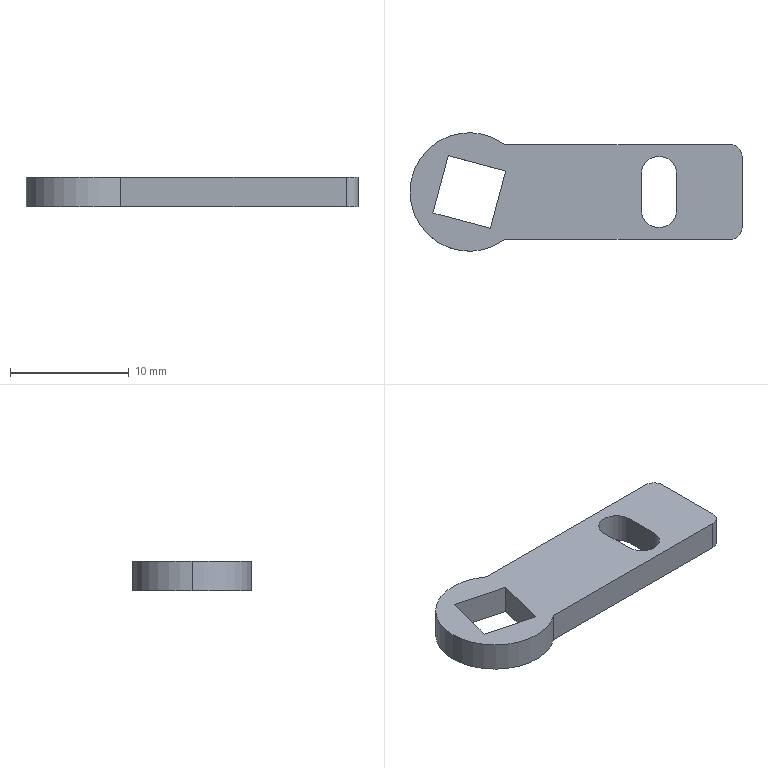Part | SolidWorks | features Extrusion 1, Fillet 1, ICE 1 | 1 solid | 17 faces | box 28 x 10 x 2.5 mm | volume 464.649 mm3 | plane 11 | cylinder 6 | commonest cylinder face diameters 2 x2 3 x2 10 x2
STEP:
#1=CARTESIAN_POINT('',(-5.,0.,1.25));
#2=VERTEX_POINT('',#1);
#3=CARTESIAN_POINT('',(3.,-4.,1.25));
#4=VERTEX_POINT('',#3);
#5=CARTESIAN_POINT('',(0.,0.,1.25));
#6=DIRECTION('',(0.,0.,1.));
#7=DIRECTION('',(1.,0.,0.));
#8=AXIS2_PLACEMENT_3D('',#5,#6,#7);
#9=CIRCLE('',#8,5.);
#10=EDGE_CURVE('',#2,#4,#9,.T.);
#11=ORIENTED_EDGE('',*,*,#10,.F.);
#12=CARTESIAN_POINT('',(-5.,0.,-1.25));
#13=VERTEX_POINT('',#12);
#14=CARTESIAN_POINT('',(-5.,0.,1.25));
#15=DIRECTION('',(0.,0.,-1.));
#16=VECTOR('',#15,1000.);
#17=LINE('',#14,#16);
#18=EDGE_CURVE('',#2,#13,#17,.T.);
#19=ORIENTED_EDGE('',*,*,#18,.T.);
#20=CARTESIAN_POINT('',(3.,-4.,-1.25));
#21=VERTEX_POINT('',#20);
#22=CARTESIAN_POINT('',(0.,0.,-1.25));
#23=DIRECTION('',(0.,0.,1.));
#24=DIRECTION('',(1.,0.,0.));
#25=AXIS2_PLACEMENT_3D('',#22,#23,#24);
#26=CIRCLE('',#25,5.);
#27=EDGE_CURVE('',#13,#21,#26,.T.);
#28=ORIENTED_EDGE('',*,*,#27,.T.);
#29=CARTESIAN_POINT('',(3.,-4.,1.25));
#30=DIRECTION('',(0.,0.,-1.));
#31=VECTOR('',#30,1000.);
#32=LINE('',#29,#31);
#33=EDGE_CURVE('',#4,#21,#32,.T.);
#34=ORIENTED_EDGE('',*,*,#33,.F.);
#35=EDGE_LOOP('',(#11,#19,#28,#34));
#36=FACE_OUTER_BOUND('',#35,.T.);
#37=CARTESIAN_POINT('',(0.,0.,1.25));
#38=DIRECTION('',(0.,0.,-1.));
#39=DIRECTION('',(-1.,0.,0.));
#40=AXIS2_PLACEMENT_3D('',#37,#38,#39);
#41=CYLINDRICAL_SURFACE('',#40,5.);
#42=ADVANCED_FACE('',(#36),#41,.T.);
#43=ORIENTED_EDGE('',*,*,#18,.F.);
#44=CARTESIAN_POINT('',(3.,4.,1.25));
#45=VERTEX_POINT('',#44);
#46=CARTESIAN_POINT('',(0.,0.,1.25));
#47=DIRECTION('',(0.,0.,1.));
#48=DIRECTION('',(1.,0.,0.));
#49=AXIS2_PLACEMENT_3D('',#46,#47,#48);
#50=CIRCLE('',#49,5.);
#51=EDGE_CURVE('',#45,#2,#50,.T.);
#52=ORIENTED_EDGE('',*,*,#51,.F.);
#53=CARTESIAN_POINT('',(3.,4.,-1.25));
#54=VERTEX_POINT('',#53);
#55=CARTESIAN_POINT('',(3.,4.,1.25));
#56=DIRECTION('',(0.,0.,-1.));
#57=VECTOR('',#56,1000.);
#58=LINE('',#55,#57);
#59=EDGE_CURVE('',#45,#54,#58,.T.);
#60=ORIENTED_EDGE('',*,*,#59,.T.);
#61=CARTESIAN_POINT('',(0.,0.,-1.25));
#62=DIRECTION('',(0.,0.,1.));
#63=DIRECTION('',(1.,0.,0.));
#64=AXIS2_PLACEMENT_3D('',#61,#62,#63);
#65=CIRCLE('',#64,5.);
#66=EDGE_CURVE('',#54,#13,#65,.T.);
#67=ORIENTED_EDGE('',*,*,#66,.T.);
#68=EDGE_LOOP('',(#43,#52,#60,#67));
#69=FACE_OUTER_BOUND('',#68,.T.);
#70=CARTESIAN_POINT('',(0.,0.,1.25));
#71=DIRECTION('',(0.,0.,-1.));
#72=DIRECTION('',(-1.,0.,0.));
#73=AXIS2_PLACEMENT_3D('',#70,#71,#72);
#74=CYLINDRICAL_SURFACE('',#73,5.);
#75=ADVANCED_FACE('',(#69),#74,.T.);
#76=CARTESIAN_POINT('',(22.,-4.,-1.25));
#77=VERTEX_POINT('',#76);
#78=CARTESIAN_POINT('',(3.,-4.,-1.25));
#79=DIRECTION('',(1.,0.,0.));
#80=VECTOR('',#79,1000.);
#81=LINE('',#78,#80);
#82=EDGE_CURVE('',#21,#77,#81,.T.);
#83=ORIENTED_EDGE('',*,*,#82,.T.);
#84=CARTESIAN_POINT('',(22.,-4.,1.25));
#85=VERTEX_POINT('',#84);
#86=CARTESIAN_POINT('',(22.,-4.,1.25));
#87=DIRECTION('',(0.,0.,1.));
#88=VECTOR('',#87,1000.);
#89=LINE('',#86,#88);
#90=EDGE_CURVE('',#77,#85,#89,.T.);
#91=ORIENTED_EDGE('',*,*,#90,.T.);
#92=CARTESIAN_POINT('',(3.,-4.,1.25));
#93=DIRECTION('',(1.,0.,0.));
#94=VECTOR('',#93,1000.);
#95=LINE('',#92,#94);
#96=EDGE_CURVE('',#4,#85,#95,.T.);
#97=ORIENTED_EDGE('',*,*,#96,.F.);
#98=ORIENTED_EDGE('',*,*,#33,.T.);
#99=EDGE_LOOP('',(#83,#91,#97,#98));
#100=FACE_OUTER_BOUND('',#99,.T.);
#101=CARTESIAN_POINT('',(3.,-4.,1.25));
#102=DIRECTION('',(0.,1.,0.));
#103=DIRECTION('',(0.,0.,1.));
#104=AXIS2_PLACEMENT_3D('',#101,#102,#103);
#105=PLANE('',#104);
#106=ADVANCED_FACE('',(#100),#105,.F.);
#107=CARTESIAN_POINT('',(23.,-3.,1.25));
#108=VERTEX_POINT('',#107);
#109=CARTESIAN_POINT('',(23.,3.,1.25));
#110=VERTEX_POINT('',#109);
#111=CARTESIAN_POINT('',(23.,4.,1.25));
#112=DIRECTION('',(0.,1.,0.));
#113=VECTOR('',#112,1000.);
#114=LINE('',#111,#113);
#115=EDGE_CURVE('',#108,#110,#114,.T.);
#116=ORIENTED_EDGE('',*,*,#115,.F.);
#117=CARTESIAN_POINT('',(23.,-3.,-1.25));
#118=VERTEX_POINT('',#117);
#119=CARTESIAN_POINT('',(23.,-3.,1.25));
#120=DIRECTION('',(0.,0.,-1.));
#121=VECTOR('',#120,1000.);
#122=LINE('',#119,#121);
#123=EDGE_CURVE('',#108,#118,#122,.T.);
#124=ORIENTED_EDGE('',*,*,#123,.T.);
#125=CARTESIAN_POINT('',(23.,3.,-1.25));
#126=VERTEX_POINT('',#125);
#127=CARTESIAN_POINT('',(23.,4.,-1.25));
#128=DIRECTION('',(0.,1.,0.));
#129=VECTOR('',#128,1000.);
#130=LINE('',#127,#129);
#131=EDGE_CURVE('',#118,#126,#130,.T.);
#132=ORIENTED_EDGE('',*,*,#131,.T.);
#133=CARTESIAN_POINT('',(23.,3.,1.25));
#134=DIRECTION('',(0.,0.,1.));
#135=VECTOR('',#134,1000.);
#136=LINE('',#133,#135);
#137=EDGE_CURVE('',#126,#110,#136,.T.);
#138=ORIENTED_EDGE('',*,*,#137,.T.);
#139=EDGE_LOOP('',(#116,#124,#132,#138));
#140=FACE_OUTER_BOUND('',#139,.T.);
#141=CARTESIAN_POINT('',(23.,4.,1.25));
#142=DIRECTION('',(-1.,0.,0.));
#143=DIRECTION('',(0.,0.,1.));
#144=AXIS2_PLACEMENT_3D('',#141,#142,#143);
#145=PLANE('',#144);
#146=ADVANCED_FACE('',(#140),#145,.F.);
#147=CARTESIAN_POINT('',(22.,4.,1.25));
#148=VERTEX_POINT('',#147);
#149=CARTESIAN_POINT('',(3.,4.,1.25));
#150=DIRECTION('',(-1.,0.,0.));
#151=VECTOR('',#150,1000.);
#152=LINE('',#149,#151);
#153=EDGE_CURVE('',#148,#45,#152,.T.);
#154=ORIENTED_EDGE('',*,*,#153,.F.);
#155=CARTESIAN_POINT('',(22.,4.,-1.25));
#156=VERTEX_POINT('',#155);
#157=CARTESIAN_POINT('',(22.,4.,1.25));
#158=DIRECTION('',(0.,0.,-1.));
#159=VECTOR('',#158,1000.);
#160=LINE('',#157,#159);
#161=EDGE_CURVE('',#148,#156,#160,.T.);
#162=ORIENTED_EDGE('',*,*,#161,.T.);
#163=CARTESIAN_POINT('',(3.,4.,-1.25));
#164=DIRECTION('',(-1.,0.,0.));
#165=VECTOR('',#164,1000.);
#166=LINE('',#163,#165);
#167=EDGE_CURVE('',#156,#54,#166,.T.);
#168=ORIENTED_EDGE('',*,*,#167,.T.);
#169=ORIENTED_EDGE('',*,*,#59,.F.);
#170=EDGE_LOOP('',(#154,#162,#168,#169));
#171=FACE_OUTER_BOUND('',#170,.T.);
#172=CARTESIAN_POINT('',(3.,4.,1.25));
#173=DIRECTION('',(0.,-1.,0.));
#174=DIRECTION('',(0.,0.,-1.));
#175=AXIS2_PLACEMENT_3D('',#172,#173,#174);
#176=PLANE('',#175);
#177=ADVANCED_FACE('',(#171),#176,.F.);
#178=CARTESIAN_POINT('',(14.5,-1.5,1.25));
#179=VERTEX_POINT('',#178);
#180=CARTESIAN_POINT('',(17.5,-1.5,1.25));
#181=VERTEX_POINT('',#180);
#182=CARTESIAN_POINT('',(16.,-1.5,1.25));
#183=DIRECTION('',(0.,0.,1.));
#184=DIRECTION('',(1.,0.,0.));
#185=AXIS2_PLACEMENT_3D('',#182,#183,#184);
#186=CIRCLE('',#185,1.5);
#187=EDGE_CURVE('',#179,#181,#186,.T.);
#188=ORIENTED_EDGE('',*,*,#187,.F.);
#189=CARTESIAN_POINT('',(14.5,1.5,1.25));
#190=VERTEX_POINT('',#189);
#191=CARTESIAN_POINT('',(14.5,-1.5,1.25));
#192=DIRECTION('',(0.,-1.,0.));
#193=VECTOR('',#192,1000.);
#194=LINE('',#191,#193);
#195=EDGE_CURVE('',#190,#179,#194,.T.);
#196=ORIENTED_EDGE('',*,*,#195,.F.);
#197=CARTESIAN_POINT('',(17.5,1.5,1.25));
#198=VERTEX_POINT('',#197);
#199=CARTESIAN_POINT('',(16.,1.5,1.25));
#200=DIRECTION('',(0.,0.,1.));
#201=DIRECTION('',(1.,0.,0.));
#202=AXIS2_PLACEMENT_3D('',#199,#200,#201);
#203=CIRCLE('',#202,1.5);
#204=EDGE_CURVE('',#198,#190,#203,.T.);
#205=ORIENTED_EDGE('',*,*,#204,.F.);
#206=CARTESIAN_POINT('',(17.5,-1.5,1.25));
#207=DIRECTION('',(0.,1.,0.));
#208=VECTOR('',#207,1000.);
#209=LINE('',#206,#208);
#210=EDGE_CURVE('',#181,#198,#209,.T.);
#211=ORIENTED_EDGE('',*,*,#210,.F.);
#212=EDGE_LOOP('',(#188,#196,#205,#211));
#213=FACE_BOUND('',#212,.T.);
#214=CARTESIAN_POINT('',(3.062,1.768,1.25));
#215=VERTEX_POINT('',#214);
#216=CARTESIAN_POINT('',(-1.768,3.062,1.25));
#217=VERTEX_POINT('',#216);
#218=CARTESIAN_POINT('',(3.062,1.768,1.25));
#219=DIRECTION('',(-0.9659,0.2588,0.));
#220=VECTOR('',#219,1000.);
#221=LINE('',#218,#220);
#222=EDGE_CURVE('',#215,#217,#221,.T.);
#223=ORIENTED_EDGE('',*,*,#222,.F.);
#224=CARTESIAN_POINT('',(1.768,-3.062,1.25));
#225=VERTEX_POINT('',#224);
#226=CARTESIAN_POINT('',(1.768,-3.062,1.25));
#227=DIRECTION('',(0.2588,0.9659,0.));
#228=VECTOR('',#227,1000.);
#229=LINE('',#226,#228);
#230=EDGE_CURVE('',#225,#215,#229,.T.);
#231=ORIENTED_EDGE('',*,*,#230,.F.);
#232=CARTESIAN_POINT('',(-3.062,-1.768,1.25));
#233=VERTEX_POINT('',#232);
#234=CARTESIAN_POINT('',(1.768,-3.062,1.25));
#235=DIRECTION('',(0.9659,-0.2588,0.));
#236=VECTOR('',#235,1000.);
#237=LINE('',#234,#236);
#238=EDGE_CURVE('',#233,#225,#237,.T.);
#239=ORIENTED_EDGE('',*,*,#238,.F.);
#240=CARTESIAN_POINT('',(-3.062,-1.768,1.25));
#241=DIRECTION('',(-0.2588,-0.9659,0.));
#242=VECTOR('',#241,1000.);
#243=LINE('',#240,#242);
#244=EDGE_CURVE('',#217,#233,#243,.T.);
#245=ORIENTED_EDGE('',*,*,#244,.F.);
#246=EDGE_LOOP('',(#223,#231,#239,#245));
#247=FACE_BOUND('',#246,.T.);
#248=ORIENTED_EDGE('',*,*,#96,.T.);
#249=CARTESIAN_POINT('',(22.,-3.,1.25));
#250=DIRECTION('',(0.,0.,1.));
#251=DIRECTION('',(1.,0.,0.));
#252=AXIS2_PLACEMENT_3D('',#249,#250,#251);
#253=CIRCLE('',#252,1.);
#254=EDGE_CURVE('',#85,#108,#253,.T.);
#255=ORIENTED_EDGE('',*,*,#254,.T.);
#256=ORIENTED_EDGE('',*,*,#115,.T.);
#257=CARTESIAN_POINT('',(22.,3.,1.25));
#258=DIRECTION('',(0.,0.,1.));
#259=DIRECTION('',(1.,0.,0.));
#260=AXIS2_PLACEMENT_3D('',#257,#258,#259);
#261=CIRCLE('',#260,1.);
#262=EDGE_CURVE('',#110,#148,#261,.T.);
#263=ORIENTED_EDGE('',*,*,#262,.T.);
#264=ORIENTED_EDGE('',*,*,#153,.T.);
#265=ORIENTED_EDGE('',*,*,#51,.T.);
#266=ORIENTED_EDGE('',*,*,#10,.T.);
#267=EDGE_LOOP('',(#248,#255,#256,#263,#264,#265,#266));
#268=FACE_OUTER_BOUND('',#267,.T.);
#269=CARTESIAN_POINT('',(0.,0.,1.25));
#270=DIRECTION('',(0.,0.,1.));
#271=DIRECTION('',(1.,0.,0.));
#272=AXIS2_PLACEMENT_3D('',#269,#270,#271);
#273=PLANE('',#272);
#274=ADVANCED_FACE('',(#213,#247,#268),#273,.T.);
#275=CARTESIAN_POINT('',(14.5,1.5,-1.25));
#276=VERTEX_POINT('',#275);
#277=CARTESIAN_POINT('',(14.5,-1.5,-1.25));
#278=VERTEX_POINT('',#277);
#279=CARTESIAN_POINT('',(14.5,-1.5,-1.25));
#280=DIRECTION('',(0.,-1.,0.));
#281=VECTOR('',#280,1000.);
#282=LINE('',#279,#281);
#283=EDGE_CURVE('',#276,#278,#282,.T.);
#284=ORIENTED_EDGE('',*,*,#283,.T.);
#285=CARTESIAN_POINT('',(17.5,-1.5,-1.25));
#286=VERTEX_POINT('',#285);
#287=CARTESIAN_POINT('',(16.,-1.5,-1.25));
#288=DIRECTION('',(0.,0.,1.));
#289=DIRECTION('',(1.,0.,0.));
#290=AXIS2_PLACEMENT_3D('',#287,#288,#289);
#291=CIRCLE('',#290,1.5);
#292=EDGE_CURVE('',#278,#286,#291,.T.);
#293=ORIENTED_EDGE('',*,*,#292,.T.);
#294=CARTESIAN_POINT('',(17.5,1.5,-1.25));
#295=VERTEX_POINT('',#294);
#296=CARTESIAN_POINT('',(17.5,-1.5,-1.25));
#297=DIRECTION('',(0.,1.,0.));
#298=VECTOR('',#297,1000.);
#299=LINE('',#296,#298);
#300=EDGE_CURVE('',#286,#295,#299,.T.);
#301=ORIENTED_EDGE('',*,*,#300,.T.);
#302=CARTESIAN_POINT('',(16.,1.5,-1.25));
#303=DIRECTION('',(0.,0.,1.));
#304=DIRECTION('',(1.,0.,0.));
#305=AXIS2_PLACEMENT_3D('',#302,#303,#304);
#306=CIRCLE('',#305,1.5);
#307=EDGE_CURVE('',#295,#276,#306,.T.);
#308=ORIENTED_EDGE('',*,*,#307,.T.);
#309=EDGE_LOOP('',(#284,#293,#301,#308));
#310=FACE_BOUND('',#309,.T.);
#311=CARTESIAN_POINT('',(1.768,-3.062,-1.25));
#312=VERTEX_POINT('',#311);
#313=CARTESIAN_POINT('',(3.062,1.768,-1.25));
#314=VERTEX_POINT('',#313);
#315=CARTESIAN_POINT('',(1.768,-3.062,-1.25));
#316=DIRECTION('',(0.2588,0.9659,0.));
#317=VECTOR('',#316,1000.);
#318=LINE('',#315,#317);
#319=EDGE_CURVE('',#312,#314,#318,.T.);
#320=ORIENTED_EDGE('',*,*,#319,.T.);
#321=CARTESIAN_POINT('',(-1.768,3.062,-1.25));
#322=VERTEX_POINT('',#321);
#323=CARTESIAN_POINT('',(3.062,1.768,-1.25));
#324=DIRECTION('',(-0.9659,0.2588,0.));
#325=VECTOR('',#324,1000.);
#326=LINE('',#323,#325);
#327=EDGE_CURVE('',#314,#322,#326,.T.);
#328=ORIENTED_EDGE('',*,*,#327,.T.);
#329=CARTESIAN_POINT('',(-3.062,-1.768,-1.25));
#330=VERTEX_POINT('',#329);
#331=CARTESIAN_POINT('',(-3.062,-1.768,-1.25));
#332=DIRECTION('',(-0.2588,-0.9659,0.));
#333=VECTOR('',#332,1000.);
#334=LINE('',#331,#333);
#335=EDGE_CURVE('',#322,#330,#334,.T.);
#336=ORIENTED_EDGE('',*,*,#335,.T.);
#337=CARTESIAN_POINT('',(1.768,-3.062,-1.25));
#338=DIRECTION('',(0.9659,-0.2588,0.));
#339=VECTOR('',#338,1000.);
#340=LINE('',#337,#339);
#341=EDGE_CURVE('',#330,#312,#340,.T.);
#342=ORIENTED_EDGE('',*,*,#341,.T.);
#343=EDGE_LOOP('',(#320,#328,#336,#342));
#344=FACE_BOUND('',#343,.T.);
#345=ORIENTED_EDGE('',*,*,#131,.F.);
#346=CARTESIAN_POINT('',(22.,-3.,-1.25));
#347=DIRECTION('',(0.,0.,-1.));
#348=DIRECTION('',(1.,0.,0.));
#349=AXIS2_PLACEMENT_3D('',#346,#347,#348);
#350=CIRCLE('',#349,1.);
#351=EDGE_CURVE('',#118,#77,#350,.T.);
#352=ORIENTED_EDGE('',*,*,#351,.T.);
#353=ORIENTED_EDGE('',*,*,#82,.F.);
#354=ORIENTED_EDGE('',*,*,#27,.F.);
#355=ORIENTED_EDGE('',*,*,#66,.F.);
#356=ORIENTED_EDGE('',*,*,#167,.F.);
#357=CARTESIAN_POINT('',(22.,3.,-1.25));
#358=DIRECTION('',(0.,0.,-1.));
#359=DIRECTION('',(1.,0.,0.));
#360=AXIS2_PLACEMENT_3D('',#357,#358,#359);
#361=CIRCLE('',#360,1.);
#362=EDGE_CURVE('',#156,#126,#361,.T.);
#363=ORIENTED_EDGE('',*,*,#362,.T.);
#364=EDGE_LOOP('',(#345,#352,#353,#354,#355,#356,#363));
#365=FACE_OUTER_BOUND('',#364,.T.);
#366=CARTESIAN_POINT('',(0.,0.,-1.25));
#367=DIRECTION('',(0.,0.,1.));
#368=DIRECTION('',(1.,0.,0.));
#369=AXIS2_PLACEMENT_3D('',#366,#367,#368);
#370=PLANE('',#369);
#371=ADVANCED_FACE('',(#310,#344,#365),#370,.F.);
#372=ORIENTED_EDGE('',*,*,#222,.T.);
#373=CARTESIAN_POINT('',(-1.768,3.062,-1.25));
#374=DIRECTION('',(0.,0.,1.));
#375=VECTOR('',#374,1000.);
#376=LINE('',#373,#375);
#377=EDGE_CURVE('',#322,#217,#376,.T.);
#378=ORIENTED_EDGE('',*,*,#377,.F.);
#379=ORIENTED_EDGE('',*,*,#327,.F.);
#380=CARTESIAN_POINT('',(3.062,1.768,-1.25));
#381=DIRECTION('',(0.,0.,1.));
#382=VECTOR('',#381,1000.);
#383=LINE('',#380,#382);
#384=EDGE_CURVE('',#314,#215,#383,.T.);
#385=ORIENTED_EDGE('',*,*,#384,.T.);
#386=EDGE_LOOP('',(#372,#378,#379,#385));
#387=FACE_OUTER_BOUND('',#386,.T.);
#388=CARTESIAN_POINT('',(3.062,1.768,-1.25));
#389=DIRECTION('',(0.2588,0.9659,0.));
#390=DIRECTION('',(-0.9659,0.2588,0.));
#391=AXIS2_PLACEMENT_3D('',#388,#389,#390);
#392=PLANE('',#391);
#393=ADVANCED_FACE('',(#387),#392,.F.);
#394=ORIENTED_EDGE('',*,*,#230,.T.);
#395=ORIENTED_EDGE('',*,*,#384,.F.);
#396=ORIENTED_EDGE('',*,*,#319,.F.);
#397=CARTESIAN_POINT('',(1.768,-3.062,-1.25));
#398=DIRECTION('',(0.,0.,1.));
#399=VECTOR('',#398,1000.);
#400=LINE('',#397,#399);
#401=EDGE_CURVE('',#312,#225,#400,.T.);
#402=ORIENTED_EDGE('',*,*,#401,.T.);
#403=EDGE_LOOP('',(#394,#395,#396,#402));
#404=FACE_OUTER_BOUND('',#403,.T.);
#405=CARTESIAN_POINT('',(1.768,-3.062,-1.25));
#406=DIRECTION('',(0.9659,-0.2588,0.));
#407=DIRECTION('',(0.2588,0.9659,0.));
#408=AXIS2_PLACEMENT_3D('',#405,#406,#407);
#409=PLANE('',#408);
#410=ADVANCED_FACE('',(#404),#409,.F.);
#411=ORIENTED_EDGE('',*,*,#238,.T.);
#412=ORIENTED_EDGE('',*,*,#401,.F.);
#413=ORIENTED_EDGE('',*,*,#341,.F.);
#414=CARTESIAN_POINT('',(-3.062,-1.768,-1.25));
#415=DIRECTION('',(0.,0.,1.));
#416=VECTOR('',#415,1000.);
#417=LINE('',#414,#416);
#418=EDGE_CURVE('',#330,#233,#417,.T.);
#419=ORIENTED_EDGE('',*,*,#418,.T.);
#420=EDGE_LOOP('',(#411,#412,#413,#419));
#421=FACE_OUTER_BOUND('',#420,.T.);
#422=CARTESIAN_POINT('',(1.768,-3.062,-1.25));
#423=DIRECTION('',(-0.2588,-0.9659,0.));
#424=DIRECTION('',(0.9659,-0.2588,0.));
#425=AXIS2_PLACEMENT_3D('',#422,#423,#424);
#426=PLANE('',#425);
#427=ADVANCED_FACE('',(#421),#426,.F.);
#428=ORIENTED_EDGE('',*,*,#244,.T.);
#429=ORIENTED_EDGE('',*,*,#418,.F.);
#430=ORIENTED_EDGE('',*,*,#335,.F.);
#431=ORIENTED_EDGE('',*,*,#377,.T.);
#432=EDGE_LOOP('',(#428,#429,#430,#431));
#433=FACE_OUTER_BOUND('',#432,.T.);
#434=CARTESIAN_POINT('',(-3.062,-1.768,-1.25));
#435=DIRECTION('',(-0.9659,0.2588,0.));
#436=DIRECTION('',(-0.2588,-0.9659,0.));
#437=AXIS2_PLACEMENT_3D('',#434,#435,#436);
#438=PLANE('',#437);
#439=ADVANCED_FACE('',(#433),#438,.F.);
#440=ORIENTED_EDGE('',*,*,#187,.T.);
#441=CARTESIAN_POINT('',(17.5,-1.5,-1.25));
#442=DIRECTION('',(0.,0.,1.));
#443=VECTOR('',#442,1000.);
#444=LINE('',#441,#443);
#445=EDGE_CURVE('',#286,#181,#444,.T.);
#446=ORIENTED_EDGE('',*,*,#445,.F.);
#447=ORIENTED_EDGE('',*,*,#292,.F.);
#448=CARTESIAN_POINT('',(14.5,-1.5,-1.25));
#449=DIRECTION('',(0.,0.,1.));
#450=VECTOR('',#449,1000.);
#451=LINE('',#448,#450);
#452=EDGE_CURVE('',#278,#179,#451,.T.);
#453=ORIENTED_EDGE('',*,*,#452,.T.);
#454=EDGE_LOOP('',(#440,#446,#447,#453));
#455=FACE_OUTER_BOUND('',#454,.T.);
#456=CARTESIAN_POINT('',(16.,-1.5,-1.25));
#457=DIRECTION('',(0.,0.,1.));
#458=DIRECTION('',(1.,0.,0.));
#459=AXIS2_PLACEMENT_3D('',#456,#457,#458);
#460=CYLINDRICAL_SURFACE('',#459,1.5);
#461=ADVANCED_FACE('',(#455),#460,.F.);
#462=ORIENTED_EDGE('',*,*,#195,.T.);
#463=ORIENTED_EDGE('',*,*,#452,.F.);
#464=ORIENTED_EDGE('',*,*,#283,.F.);
#465=CARTESIAN_POINT('',(14.5,1.5,-1.25));
#466=DIRECTION('',(0.,0.,1.));
#467=VECTOR('',#466,1000.);
#468=LINE('',#465,#467);
#469=EDGE_CURVE('',#276,#190,#468,.T.);
#470=ORIENTED_EDGE('',*,*,#469,.T.);
#471=EDGE_LOOP('',(#462,#463,#464,#470));
#472=FACE_OUTER_BOUND('',#471,.T.);
#473=CARTESIAN_POINT('',(14.5,-1.5,-1.25));
#474=DIRECTION('',(-1.,0.,0.));
#475=DIRECTION('',(0.,0.,1.));
#476=AXIS2_PLACEMENT_3D('',#473,#474,#475);
#477=PLANE('',#476);
#478=ADVANCED_FACE('',(#472),#477,.F.);
#479=ORIENTED_EDGE('',*,*,#204,.T.);
#480=ORIENTED_EDGE('',*,*,#469,.F.);
#481=ORIENTED_EDGE('',*,*,#307,.F.);
#482=CARTESIAN_POINT('',(17.5,1.5,-1.25));
#483=DIRECTION('',(0.,0.,1.));
#484=VECTOR('',#483,1000.);
#485=LINE('',#482,#484);
#486=EDGE_CURVE('',#295,#198,#485,.T.);
#487=ORIENTED_EDGE('',*,*,#486,.T.);
#488=EDGE_LOOP('',(#479,#480,#481,#487));
#489=FACE_OUTER_BOUND('',#488,.T.);
#490=CARTESIAN_POINT('',(16.,1.5,-1.25));
#491=DIRECTION('',(0.,0.,1.));
#492=DIRECTION('',(1.,0.,0.));
#493=AXIS2_PLACEMENT_3D('',#490,#491,#492);
#494=CYLINDRICAL_SURFACE('',#493,1.5);
#495=ADVANCED_FACE('',(#489),#494,.F.);
#496=ORIENTED_EDGE('',*,*,#210,.T.);
#497=ORIENTED_EDGE('',*,*,#486,.F.);
#498=ORIENTED_EDGE('',*,*,#300,.F.);
#499=ORIENTED_EDGE('',*,*,#445,.T.);
#500=EDGE_LOOP('',(#496,#497,#498,#499));
#501=FACE_OUTER_BOUND('',#500,.T.);
#502=CARTESIAN_POINT('',(17.5,-1.5,-1.25));
#503=DIRECTION('',(1.,0.,0.));
#504=DIRECTION('',(0.,0.,-1.));
#505=AXIS2_PLACEMENT_3D('',#502,#503,#504);
#506=PLANE('',#505);
#507=ADVANCED_FACE('',(#501),#506,.F.);
#508=ORIENTED_EDGE('',*,*,#254,.F.);
#509=ORIENTED_EDGE('',*,*,#90,.F.);
#510=ORIENTED_EDGE('',*,*,#351,.F.);
#511=ORIENTED_EDGE('',*,*,#123,.F.);
#512=EDGE_LOOP('',(#508,#509,#510,#511));
#513=FACE_OUTER_BOUND('',#512,.T.);
#514=CARTESIAN_POINT('',(22.,-3.,1.25));
#515=DIRECTION('',(0.,0.,-1.));
#516=DIRECTION('',(-1.,0.,0.));
#517=AXIS2_PLACEMENT_3D('',#514,#515,#516);
#518=CYLINDRICAL_SURFACE('',#517,1.);
#519=ADVANCED_FACE('',(#513),#518,.T.);
#520=ORIENTED_EDGE('',*,*,#262,.F.);
#521=ORIENTED_EDGE('',*,*,#137,.F.);
#522=ORIENTED_EDGE('',*,*,#362,.F.);
#523=ORIENTED_EDGE('',*,*,#161,.F.);
#524=EDGE_LOOP('',(#520,#521,#522,#523));
#525=FACE_OUTER_BOUND('',#524,.T.);
#526=CARTESIAN_POINT('',(22.,3.,1.25));
#527=DIRECTION('',(0.,0.,-1.));
#528=DIRECTION('',(-1.,0.,0.));
#529=AXIS2_PLACEMENT_3D('',#526,#527,#528);
#530=CYLINDRICAL_SURFACE('',#529,1.);
#531=ADVANCED_FACE('',(#525),#530,.T.);
#532=CLOSED_SHELL('',(#42,#75,#106,#146,#177,#274,#371,#393,#410,#427,#439,#461,#478,#495,#507,#519,#531));
#533=MANIFOLD_SOLID_BREP('',#532);
#534=CARTESIAN_POINT('',(0.,0.,0.));
#535=DIRECTION('',(0.,0.,1.));
#536=DIRECTION('',(1.,0.,0.));
#537=AXIS2_PLACEMENT_3D('',#534,#535,#536);
#538=(LENGTH_UNIT()NAMED_UNIT(*)SI_UNIT(.MILLI.,.METRE.));
#539=UNCERTAINTY_MEASURE_WITH_UNIT(LENGTH_MEASURE(0.00001),#538,'','');
#540=(NAMED_UNIT(*)PLANE_ANGLE_UNIT()SI_UNIT($,.RADIAN.));
#541=(NAMED_UNIT(*)SI_UNIT($,.STERADIAN.)SOLID_ANGLE_UNIT());
#542=(GEOMETRIC_REPRESENTATION_CONTEXT(3)GLOBAL_UNCERTAINTY_ASSIGNED_CONTEXT((#539))GLOBAL_UNIT_ASSIGNED_CONTEXT((#538,#540,#541))REPRESENTATION_CONTEXT('',''));
#543=ADVANCED_BREP_SHAPE_REPRESENTATION('',(#533,#537),#542);